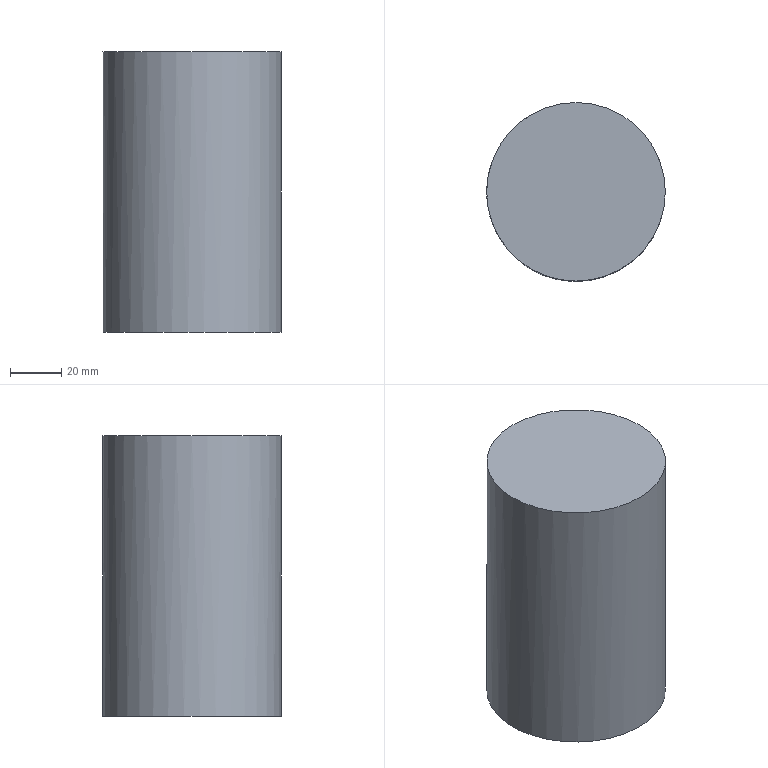Part | NX | features solid 2 | 1 solid | 3 faces | box 70 x 70 x 110 mm | volume 423330 mm3 | plane 2 | cylinder 1 | commonest cylinder face diameters 70 x1
STEP:
#1=CARTESIAN_POINT('',(-1550.,570.,95.));
#2=VERTEX_POINT('',#1);
#3=CARTESIAN_POINT('',(-1515.,570.,95.));
#4=DIRECTION('',(0.,0.,1.));
#5=DIRECTION('',(-1.,0.,0.));
#6=AXIS2_PLACEMENT_3D('',#3,#4,#5);
#7=CIRCLE('',#6,35.);
#8=EDGE_CURVE('',#2,#2,#7,.T.);
#9=ORIENTED_EDGE('',*,*,#8,.T.);
#10=EDGE_LOOP('',(#9));
#11=FACE_BOUND('',#10,.T.);
#12=CARTESIAN_POINT('',(-1515.,570.,95.));
#13=DIRECTION('',(0.,0.,1.));
#14=DIRECTION('',(1.,0.,0.));
#15=AXIS2_PLACEMENT_3D('',#12,#13,#14);
#16=PLANE('',#15);
#17=ADVANCED_FACE('',(#11),#16,.T.);
#18=CARTESIAN_POINT('',(-1480.,570.,-15.));
#19=VERTEX_POINT('',#18);
#20=CARTESIAN_POINT('',(-1515.,570.,-15.));
#21=DIRECTION('',(0.,0.,-1.));
#22=DIRECTION('',(1.,0.,0.));
#23=AXIS2_PLACEMENT_3D('',#20,#21,#22);
#24=CIRCLE('',#23,35.);
#25=EDGE_CURVE('',#19,#19,#24,.T.);
#26=ORIENTED_EDGE('',*,*,#25,.T.);
#27=EDGE_LOOP('',(#26));
#28=FACE_BOUND('',#27,.T.);
#29=CARTESIAN_POINT('',(-1515.,570.,-15.));
#30=DIRECTION('',(0.,0.,-1.));
#31=DIRECTION('',(-1.,0.,0.));
#32=AXIS2_PLACEMENT_3D('',#29,#30,#31);
#33=PLANE('',#32);
#34=ADVANCED_FACE('',(#28),#33,.T.);
#35=ORIENTED_EDGE('',*,*,#8,.F.);
#36=EDGE_LOOP('',(#35));
#37=FACE_BOUND('',#36,.T.);
#38=ORIENTED_EDGE('',*,*,#25,.F.);
#39=EDGE_LOOP('',(#38));
#40=FACE_BOUND('',#39,.T.);
#41=CARTESIAN_POINT('',(-1515.,570.,-15.));
#42=DIRECTION('',(0.,0.,1.));
#43=DIRECTION('',(1.,0.,0.));
#44=AXIS2_PLACEMENT_3D('',#41,#42,#43);
#45=CYLINDRICAL_SURFACE('',#44,35.);
#46=ADVANCED_FACE('',(#37,#40),#45,.T.);
#47=CLOSED_SHELL('',(#17,#34,#46));
#48=MANIFOLD_SOLID_BREP('',#47);
#49=(LENGTH_UNIT()NAMED_UNIT(*)SI_UNIT(.MILLI.,.METRE.));
#50=UNCERTAINTY_MEASURE_WITH_UNIT(LENGTH_MEASURE(0.00001),#49,'','');
#51=(NAMED_UNIT(*)PLANE_ANGLE_UNIT()SI_UNIT($,.RADIAN.));
#52=(NAMED_UNIT(*)SI_UNIT($,.STERADIAN.)SOLID_ANGLE_UNIT());
#53=(GEOMETRIC_REPRESENTATION_CONTEXT(3)GLOBAL_UNCERTAINTY_ASSIGNED_CONTEXT((#50))GLOBAL_UNIT_ASSIGNED_CONTEXT((#49,#51,#52))REPRESENTATION_CONTEXT('',''));
#54=ADVANCED_BREP_SHAPE_REPRESENTATION('',(#48),#53);